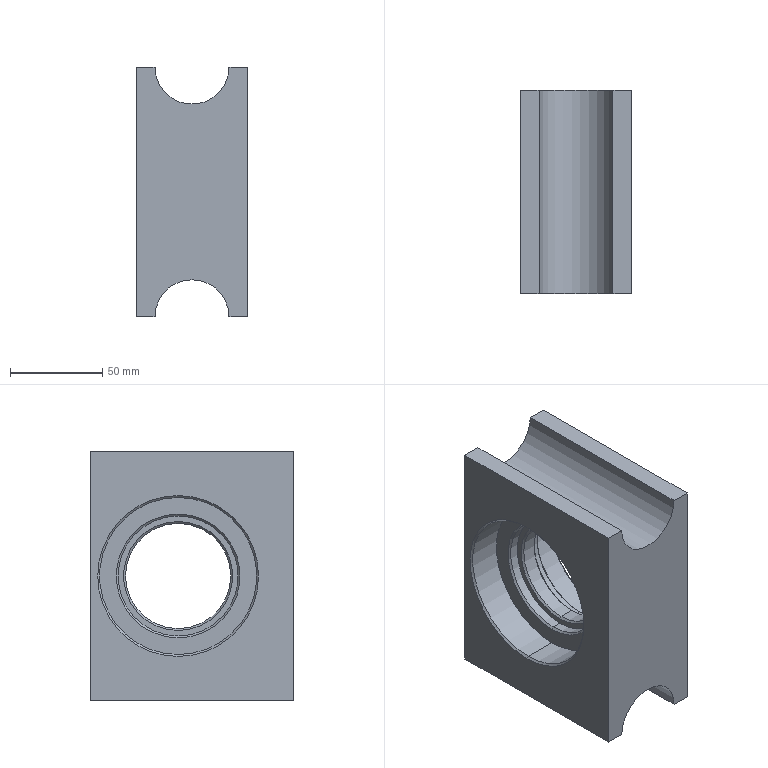Part | SolidWorks | features BaseBody 1 | 1 solid | 37 faces | box 60 x 110 x 135 mm | volume 471145 mm3 | cylinder 13 | cone 12 | plane 12 | commonest cylinder face diameters 65 x4 85 x4 40 x3 57 x2
STEP:
#1=CARTESIAN_POINT('',(0.,-55.,-47.5));
#2=VERTEX_POINT('',#1);
#3=CARTESIAN_POINT('',(20.,-55.,-67.5));
#4=VERTEX_POINT('',#3);
#5=CARTESIAN_POINT('',(0.,-55.,-67.5));
#6=DIRECTION('',(0.,1.,0.));
#7=DIRECTION('',(0.,0.,1.));
#8=AXIS2_PLACEMENT_3D('',#5,#6,#7);
#9=CIRCLE('',#8,20.);
#10=EDGE_CURVE('',#2,#4,#9,.T.);
#11=ORIENTED_EDGE('',*,*,#10,.F.);
#12=CARTESIAN_POINT('',(0.,55.,-47.5));
#13=VERTEX_POINT('',#12);
#14=CARTESIAN_POINT('',(0.,-55.,-47.5));
#15=DIRECTION('',(0.,1.,0.));
#16=VECTOR('',#15,1000.);
#17=LINE('',#14,#16);
#18=EDGE_CURVE('',#2,#13,#17,.T.);
#19=ORIENTED_EDGE('',*,*,#18,.T.);
#20=CARTESIAN_POINT('',(20.,55.,-67.5));
#21=VERTEX_POINT('',#20);
#22=CARTESIAN_POINT('',(0.,55.,-67.5));
#23=DIRECTION('',(0.,1.,0.));
#24=DIRECTION('',(0.,0.,1.));
#25=AXIS2_PLACEMENT_3D('',#22,#23,#24);
#26=CIRCLE('',#25,20.);
#27=EDGE_CURVE('',#13,#21,#26,.T.);
#28=ORIENTED_EDGE('',*,*,#27,.T.);
#29=CARTESIAN_POINT('',(20.,-55.,-67.5));
#30=DIRECTION('',(0.,1.,0.));
#31=VECTOR('',#30,1000.);
#32=LINE('',#29,#31);
#33=EDGE_CURVE('',#4,#21,#32,.T.);
#34=ORIENTED_EDGE('',*,*,#33,.F.);
#35=EDGE_LOOP('',(#11,#19,#28,#34));
#36=FACE_OUTER_BOUND('',#35,.T.);
#37=CARTESIAN_POINT('',(0.,-55.,-67.5));
#38=DIRECTION('',(0.,1.,0.));
#39=DIRECTION('',(0.,0.,1.));
#40=AXIS2_PLACEMENT_3D('',#37,#38,#39);
#41=CYLINDRICAL_SURFACE('',#40,20.);
#42=ADVANCED_FACE('',(#36),#41,.F.);
#43=CARTESIAN_POINT('',(29.,7.5,42.5));
#44=VERTEX_POINT('',#43);
#45=CARTESIAN_POINT('',(29.,7.5,-42.5));
#46=VERTEX_POINT('',#45);
#47=CARTESIAN_POINT('',(29.,7.5,0.));
#48=DIRECTION('',(1.,0.,0.));
#49=DIRECTION('',(0.,0.,-1.));
#50=AXIS2_PLACEMENT_3D('',#47,#48,#49);
#51=CIRCLE('',#50,42.5);
#52=EDGE_CURVE('',#44,#46,#51,.T.);
#53=ORIENTED_EDGE('',*,*,#52,.F.);
#54=CARTESIAN_POINT('',(30.,7.5,43.5));
#55=VERTEX_POINT('',#54);
#56=CARTESIAN_POINT('',(29.,7.5,42.5));
#57=DIRECTION('',(0.7071,0.,0.7071));
#58=VECTOR('',#57,1000.);
#59=LINE('',#56,#58);
#60=EDGE_CURVE('',#44,#55,#59,.T.);
#61=ORIENTED_EDGE('',*,*,#60,.T.);
#62=CARTESIAN_POINT('',(30.,7.5,-43.5));
#63=VERTEX_POINT('',#62);
#64=CARTESIAN_POINT('',(30.,7.5,0.));
#65=DIRECTION('',(-1.,0.,0.));
#66=DIRECTION('',(0.,0.,-1.));
#67=AXIS2_PLACEMENT_3D('',#64,#65,#66);
#68=CIRCLE('',#67,43.5);
#69=EDGE_CURVE('',#63,#55,#68,.T.);
#70=ORIENTED_EDGE('',*,*,#69,.F.);
#71=CARTESIAN_POINT('',(29.,7.5,-42.5));
#72=DIRECTION('',(0.7071,0.,-0.7071));
#73=VECTOR('',#72,1000.);
#74=LINE('',#71,#73);
#75=EDGE_CURVE('',#46,#63,#74,.T.);
#76=ORIENTED_EDGE('',*,*,#75,.F.);
#77=EDGE_LOOP('',(#53,#61,#70,#76));
#78=FACE_OUTER_BOUND('',#77,.T.);
#79=CARTESIAN_POINT('',(29.,7.5,0.));
#80=DIRECTION('',(1.,0.,0.));
#81=DIRECTION('',(0.,0.,-1.));
#82=AXIS2_PLACEMENT_3D('',#79,#80,#81);
#83=CONICAL_SURFACE('',#82,42.5,0.7854);
#84=ADVANCED_FACE('',(#78),#83,.F.);
#85=CARTESIAN_POINT('',(10.,7.5,32.5));
#86=VERTEX_POINT('',#85);
#87=CARTESIAN_POINT('',(10.,7.5,-32.5));
#88=VERTEX_POINT('',#87);
#89=CARTESIAN_POINT('',(10.,7.5,0.));
#90=DIRECTION('',(1.,0.,0.));
#91=DIRECTION('',(0.,0.,-1.));
#92=AXIS2_PLACEMENT_3D('',#89,#90,#91);
#93=CIRCLE('',#92,32.5);
#94=EDGE_CURVE('',#86,#88,#93,.T.);
#95=ORIENTED_EDGE('',*,*,#94,.F.);
#96=CARTESIAN_POINT('',(11.,7.5,33.5));
#97=VERTEX_POINT('',#96);
#98=CARTESIAN_POINT('',(10.,7.5,32.5));
#99=DIRECTION('',(0.7071,0.,0.7071));
#100=VECTOR('',#99,1000.);
#101=LINE('',#98,#100);
#102=EDGE_CURVE('',#86,#97,#101,.T.);
#103=ORIENTED_EDGE('',*,*,#102,.T.);
#104=CARTESIAN_POINT('',(11.,7.5,-33.5));
#105=VERTEX_POINT('',#104);
#106=CARTESIAN_POINT('',(11.,7.5,0.));
#107=DIRECTION('',(-1.,0.,0.));
#108=DIRECTION('',(0.,0.,-1.));
#109=AXIS2_PLACEMENT_3D('',#106,#107,#108);
#110=CIRCLE('',#109,33.5);
#111=EDGE_CURVE('',#105,#97,#110,.T.);
#112=ORIENTED_EDGE('',*,*,#111,.F.);
#113=CARTESIAN_POINT('',(10.,7.5,-32.5));
#114=DIRECTION('',(0.7071,0.,-0.7071));
#115=VECTOR('',#114,1000.);
#116=LINE('',#113,#115);
#117=EDGE_CURVE('',#88,#105,#116,.T.);
#118=ORIENTED_EDGE('',*,*,#117,.F.);
#119=EDGE_LOOP('',(#95,#103,#112,#118));
#120=FACE_OUTER_BOUND('',#119,.T.);
#121=CARTESIAN_POINT('',(10.,7.5,0.));
#122=DIRECTION('',(1.,0.,0.));
#123=DIRECTION('',(0.,0.,-1.));
#124=AXIS2_PLACEMENT_3D('',#121,#122,#123);
#125=CONICAL_SURFACE('',#124,32.5,0.7854);
#126=ADVANCED_FACE('',(#120),#125,.F.);
#127=CARTESIAN_POINT('',(4.,7.5,28.5));
#128=VERTEX_POINT('',#127);
#129=CARTESIAN_POINT('',(4.,7.5,-28.5));
#130=VERTEX_POINT('',#129);
#131=CARTESIAN_POINT('',(4.,7.5,0.));
#132=DIRECTION('',(1.,0.,0.));
#133=DIRECTION('',(0.,0.,-1.));
#134=AXIS2_PLACEMENT_3D('',#131,#132,#133);
#135=CIRCLE('',#134,28.5);
#136=EDGE_CURVE('',#128,#130,#135,.T.);
#137=ORIENTED_EDGE('',*,*,#136,.F.);
#138=CARTESIAN_POINT('',(5.,7.5,29.5));
#139=VERTEX_POINT('',#138);
#140=CARTESIAN_POINT('',(4.,7.5,28.5));
#141=DIRECTION('',(0.7071,0.,0.7071));
#142=VECTOR('',#141,1000.);
#143=LINE('',#140,#142);
#144=EDGE_CURVE('',#128,#139,#143,.T.);
#145=ORIENTED_EDGE('',*,*,#144,.T.);
#146=CARTESIAN_POINT('',(5.,7.5,-29.5));
#147=VERTEX_POINT('',#146);
#148=CARTESIAN_POINT('',(5.,7.5,0.));
#149=DIRECTION('',(-1.,0.,0.));
#150=DIRECTION('',(0.,0.,-1.));
#151=AXIS2_PLACEMENT_3D('',#148,#149,#150);
#152=CIRCLE('',#151,29.5);
#153=EDGE_CURVE('',#147,#139,#152,.T.);
#154=ORIENTED_EDGE('',*,*,#153,.F.);
#155=CARTESIAN_POINT('',(4.,7.5,-28.5));
#156=DIRECTION('',(0.7071,0.,-0.7071));
#157=VECTOR('',#156,1000.);
#158=LINE('',#155,#157);
#159=EDGE_CURVE('',#130,#147,#158,.T.);
#160=ORIENTED_EDGE('',*,*,#159,.F.);
#161=EDGE_LOOP('',(#137,#145,#154,#160));
#162=FACE_OUTER_BOUND('',#161,.T.);
#163=CARTESIAN_POINT('',(4.,7.5,0.));
#164=DIRECTION('',(1.,0.,0.));
#165=DIRECTION('',(0.,0.,-1.));
#166=AXIS2_PLACEMENT_3D('',#163,#164,#165);
#167=CONICAL_SURFACE('',#166,28.5,0.7854);
#168=ADVANCED_FACE('',(#162),#167,.F.);
#169=CARTESIAN_POINT('',(-4.,7.5,-28.5));
#170=VERTEX_POINT('',#169);
#171=CARTESIAN_POINT('',(-4.,7.5,28.5));
#172=VERTEX_POINT('',#171);
#173=CARTESIAN_POINT('',(-4.,7.5,0.));
#174=DIRECTION('',(-1.,0.,0.));
#175=DIRECTION('',(0.,0.,1.));
#176=AXIS2_PLACEMENT_3D('',#173,#174,#175);
#177=CIRCLE('',#176,28.5);
#178=EDGE_CURVE('',#170,#172,#177,.T.);
#179=ORIENTED_EDGE('',*,*,#178,.F.);
#180=CARTESIAN_POINT('',(-5.,7.5,-29.5));
#181=VERTEX_POINT('',#180);
#182=CARTESIAN_POINT('',(-4.,7.5,-28.5));
#183=DIRECTION('',(-0.7071,0.,-0.7071));
#184=VECTOR('',#183,1000.);
#185=LINE('',#182,#184);
#186=EDGE_CURVE('',#170,#181,#185,.T.);
#187=ORIENTED_EDGE('',*,*,#186,.T.);
#188=CARTESIAN_POINT('',(-5.,7.5,29.5));
#189=VERTEX_POINT('',#188);
#190=CARTESIAN_POINT('',(-5.,7.5,0.));
#191=DIRECTION('',(1.,0.,0.));
#192=DIRECTION('',(0.,0.,1.));
#193=AXIS2_PLACEMENT_3D('',#190,#191,#192);
#194=CIRCLE('',#193,29.5);
#195=EDGE_CURVE('',#189,#181,#194,.T.);
#196=ORIENTED_EDGE('',*,*,#195,.F.);
#197=CARTESIAN_POINT('',(-4.,7.5,28.5));
#198=DIRECTION('',(-0.7071,0.,0.7071));
#199=VECTOR('',#198,1000.);
#200=LINE('',#197,#199);
#201=EDGE_CURVE('',#172,#189,#200,.T.);
#202=ORIENTED_EDGE('',*,*,#201,.F.);
#203=EDGE_LOOP('',(#179,#187,#196,#202));
#204=FACE_OUTER_BOUND('',#203,.T.);
#205=CARTESIAN_POINT('',(-4.,7.5,0.));
#206=DIRECTION('',(-1.,0.,0.));
#207=DIRECTION('',(0.,0.,1.));
#208=AXIS2_PLACEMENT_3D('',#205,#206,#207);
#209=CONICAL_SURFACE('',#208,28.5,0.7854);
#210=ADVANCED_FACE('',(#204),#209,.F.);
#211=CARTESIAN_POINT('',(-10.,7.5,-32.5));
#212=VERTEX_POINT('',#211);
#213=CARTESIAN_POINT('',(-10.,7.5,32.5));
#214=VERTEX_POINT('',#213);
#215=CARTESIAN_POINT('',(-10.,7.5,0.));
#216=DIRECTION('',(-1.,0.,0.));
#217=DIRECTION('',(0.,0.,1.));
#218=AXIS2_PLACEMENT_3D('',#215,#216,#217);
#219=CIRCLE('',#218,32.5);
#220=EDGE_CURVE('',#212,#214,#219,.T.);
#221=ORIENTED_EDGE('',*,*,#220,.F.);
#222=CARTESIAN_POINT('',(-11.,7.5,-33.5));
#223=VERTEX_POINT('',#222);
#224=CARTESIAN_POINT('',(-11.,7.5,-33.5));
#225=DIRECTION('',(-0.7071,0.,-0.7071));
#226=VECTOR('',#225,1000.);
#227=LINE('',#224,#226);
#228=EDGE_CURVE('',#212,#223,#227,.T.);
#229=ORIENTED_EDGE('',*,*,#228,.T.);
#230=CARTESIAN_POINT('',(-11.,7.5,33.5));
#231=VERTEX_POINT('',#230);
#232=CARTESIAN_POINT('',(-11.,7.5,0.));
#233=DIRECTION('',(1.,0.,0.));
#234=DIRECTION('',(0.,0.,1.));
#235=AXIS2_PLACEMENT_3D('',#232,#233,#234);
#236=CIRCLE('',#235,33.5);
#237=EDGE_CURVE('',#231,#223,#236,.T.);
#238=ORIENTED_EDGE('',*,*,#237,.F.);
#239=CARTESIAN_POINT('',(-11.,7.5,33.5));
#240=DIRECTION('',(-0.7071,0.,0.7071));
#241=VECTOR('',#240,1000.);
#242=LINE('',#239,#241);
#243=EDGE_CURVE('',#214,#231,#242,.T.);
#244=ORIENTED_EDGE('',*,*,#243,.F.);
#245=EDGE_LOOP('',(#221,#229,#238,#244));
#246=FACE_OUTER_BOUND('',#245,.T.);
#247=CARTESIAN_POINT('',(-11.,7.5,0.));
#248=DIRECTION('',(-1.,0.,0.));
#249=DIRECTION('',(0.,0.,1.));
#250=AXIS2_PLACEMENT_3D('',#247,#248,#249);
#251=CONICAL_SURFACE('',#250,33.5,0.7854);
#252=ADVANCED_FACE('',(#246),#251,.F.);
#253=CARTESIAN_POINT('',(-29.,7.5,-42.5));
#254=VERTEX_POINT('',#253);
#255=CARTESIAN_POINT('',(-29.,7.5,42.5));
#256=VERTEX_POINT('',#255);
#257=CARTESIAN_POINT('',(-29.,7.5,0.));
#258=DIRECTION('',(-1.,0.,0.));
#259=DIRECTION('',(0.,0.,-1.));
#260=AXIS2_PLACEMENT_3D('',#257,#258,#259);
#261=CIRCLE('',#260,42.5);
#262=EDGE_CURVE('',#254,#256,#261,.T.);
#263=ORIENTED_EDGE('',*,*,#262,.F.);
#264=CARTESIAN_POINT('',(-30.,7.5,-43.5));
#265=VERTEX_POINT('',#264);
#266=CARTESIAN_POINT('',(-30.,7.5,-43.5));
#267=DIRECTION('',(-0.7071,0.,-0.7071));
#268=VECTOR('',#267,1000.);
#269=LINE('',#266,#268);
#270=EDGE_CURVE('',#254,#265,#269,.T.);
#271=ORIENTED_EDGE('',*,*,#270,.T.);
#272=CARTESIAN_POINT('',(-30.,7.5,43.5));
#273=VERTEX_POINT('',#272);
#274=CARTESIAN_POINT('',(-30.,7.5,0.));
#275=DIRECTION('',(1.,0.,0.));
#276=DIRECTION('',(0.,0.,-1.));
#277=AXIS2_PLACEMENT_3D('',#274,#275,#276);
#278=CIRCLE('',#277,43.5);
#279=EDGE_CURVE('',#273,#265,#278,.T.);
#280=ORIENTED_EDGE('',*,*,#279,.F.);
#281=CARTESIAN_POINT('',(-30.,7.5,43.5));
#282=DIRECTION('',(-0.7071,0.,0.7071));
#283=VECTOR('',#282,1000.);
#284=LINE('',#281,#283);
#285=EDGE_CURVE('',#256,#273,#284,.T.);
#286=ORIENTED_EDGE('',*,*,#285,.F.);
#287=EDGE_LOOP('',(#263,#271,#280,#286));
#288=FACE_OUTER_BOUND('',#287,.T.);
#289=CARTESIAN_POINT('',(-30.,7.5,0.));
#290=DIRECTION('',(-1.,0.,0.));
#291=DIRECTION('',(0.,0.,1.));
#292=AXIS2_PLACEMENT_3D('',#289,#290,#291);
#293=CONICAL_SURFACE('',#292,43.5,0.7854);
#294=ADVANCED_FACE('',(#288),#293,.F.);
#295=CARTESIAN_POINT('',(-5.,7.5,32.5));
#296=VERTEX_POINT('',#295);
#297=CARTESIAN_POINT('',(-5.,7.5,-32.5));
#298=VERTEX_POINT('',#297);
#299=CARTESIAN_POINT('',(-5.,7.5,0.));
#300=DIRECTION('',(1.,0.,0.));
#301=DIRECTION('',(0.,0.,-1.));
#302=AXIS2_PLACEMENT_3D('',#299,#300,#301);
#303=CIRCLE('',#302,32.5);
#304=EDGE_CURVE('',#296,#298,#303,.T.);
#305=ORIENTED_EDGE('',*,*,#304,.T.);
#306=CARTESIAN_POINT('',(-5.,7.5,-32.5));
#307=DIRECTION('',(-1.,0.,0.));
#308=VECTOR('',#307,1000.);
#309=LINE('',#306,#308);
#310=EDGE_CURVE('',#298,#212,#309,.T.);
#311=ORIENTED_EDGE('',*,*,#310,.T.);
#312=ORIENTED_EDGE('',*,*,#220,.T.);
#313=CARTESIAN_POINT('',(-5.,7.5,32.5));
#314=DIRECTION('',(-1.,0.,0.));
#315=VECTOR('',#314,1000.);
#316=LINE('',#313,#315);
#317=EDGE_CURVE('',#296,#214,#316,.T.);
#318=ORIENTED_EDGE('',*,*,#317,.F.);
#319=EDGE_LOOP('',(#305,#311,#312,#318));
#320=FACE_OUTER_BOUND('',#319,.T.);
#321=CARTESIAN_POINT('',(-5.,7.5,0.));
#322=DIRECTION('',(-1.,0.,0.));
#323=DIRECTION('',(0.,0.,1.));
#324=AXIS2_PLACEMENT_3D('',#321,#322,#323);
#325=CYLINDRICAL_SURFACE('',#324,32.5);
#326=ADVANCED_FACE('',(#320),#325,.F.);
#327=CARTESIAN_POINT('',(-11.,7.5,42.5));
#328=VERTEX_POINT('',#327);
#329=CARTESIAN_POINT('',(-11.,7.5,-42.5));
#330=VERTEX_POINT('',#329);
#331=CARTESIAN_POINT('',(-11.,7.5,0.));
#332=DIRECTION('',(1.,0.,0.));
#333=DIRECTION('',(0.,0.,-1.));
#334=AXIS2_PLACEMENT_3D('',#331,#332,#333);
#335=CIRCLE('',#334,42.5);
#336=EDGE_CURVE('',#328,#330,#335,.T.);
#337=ORIENTED_EDGE('',*,*,#336,.T.);
#338=CARTESIAN_POINT('',(-11.,7.5,-42.5));
#339=DIRECTION('',(-1.,0.,0.));
#340=VECTOR('',#339,1000.);
#341=LINE('',#338,#340);
#342=EDGE_CURVE('',#330,#254,#341,.T.);
#343=ORIENTED_EDGE('',*,*,#342,.T.);
#344=ORIENTED_EDGE('',*,*,#262,.T.);
#345=CARTESIAN_POINT('',(-11.,7.5,42.5));
#346=DIRECTION('',(-1.,0.,0.));
#347=VECTOR('',#346,1000.);
#348=LINE('',#345,#347);
#349=EDGE_CURVE('',#328,#256,#348,.T.);
#350=ORIENTED_EDGE('',*,*,#349,.F.);
#351=EDGE_LOOP('',(#337,#343,#344,#350));
#352=FACE_OUTER_BOUND('',#351,.T.);
#353=CARTESIAN_POINT('',(-11.,7.5,0.));
#354=DIRECTION('',(-1.,0.,0.));
#355=DIRECTION('',(0.,0.,1.));
#356=AXIS2_PLACEMENT_3D('',#353,#354,#355);
#357=CYLINDRICAL_SURFACE('',#356,42.5);
#358=ADVANCED_FACE('',(#352),#357,.F.);
#359=CARTESIAN_POINT('',(5.,7.5,32.5));
#360=VERTEX_POINT('',#359);
#361=CARTESIAN_POINT('',(5.,7.5,-32.5));
#362=VERTEX_POINT('',#361);
#363=CARTESIAN_POINT('',(5.,7.5,0.));
#364=DIRECTION('',(1.,0.,0.));
#365=DIRECTION('',(0.,0.,-1.));
#366=AXIS2_PLACEMENT_3D('',#363,#364,#365);
#367=CIRCLE('',#366,32.5);
#368=EDGE_CURVE('',#360,#362,#367,.T.);
#369=ORIENTED_EDGE('',*,*,#368,.F.);
#370=CARTESIAN_POINT('',(5.,7.5,32.5));
#371=DIRECTION('',(1.,0.,0.));
#372=VECTOR('',#371,1000.);
#373=LINE('',#370,#372);
#374=EDGE_CURVE('',#360,#86,#373,.T.);
#375=ORIENTED_EDGE('',*,*,#374,.T.);
#376=ORIENTED_EDGE('',*,*,#94,.T.);
#377=CARTESIAN_POINT('',(5.,7.5,-32.5));
#378=DIRECTION('',(1.,0.,0.));
#379=VECTOR('',#378,1000.);
#380=LINE('',#377,#379);
#381=EDGE_CURVE('',#362,#88,#380,.T.);
#382=ORIENTED_EDGE('',*,*,#381,.F.);
#383=EDGE_LOOP('',(#369,#375,#376,#382));
#384=FACE_OUTER_BOUND('',#383,.T.);
#385=CARTESIAN_POINT('',(5.,7.5,0.));
#386=DIRECTION('',(1.,0.,0.));
#387=DIRECTION('',(0.,0.,-1.));
#388=AXIS2_PLACEMENT_3D('',#385,#386,#387);
#389=CYLINDRICAL_SURFACE('',#388,32.5);
#390=ADVANCED_FACE('',(#384),#389,.F.);
#391=CARTESIAN_POINT('',(11.,7.5,42.5));
#392=VERTEX_POINT('',#391);
#393=CARTESIAN_POINT('',(11.,7.5,-42.5));
#394=VERTEX_POINT('',#393);
#395=CARTESIAN_POINT('',(11.,7.5,0.));
#396=DIRECTION('',(1.,0.,0.));
#397=DIRECTION('',(0.,0.,-1.));
#398=AXIS2_PLACEMENT_3D('',#395,#396,#397);
#399=CIRCLE('',#398,42.5);
#400=EDGE_CURVE('',#392,#394,#399,.T.);
#401=ORIENTED_EDGE('',*,*,#400,.F.);
#402=CARTESIAN_POINT('',(11.,7.5,42.5));
#403=DIRECTION('',(1.,0.,0.));
#404=VECTOR('',#403,1000.);
#405=LINE('',#402,#404);
#406=EDGE_CURVE('',#392,#44,#405,.T.);
#407=ORIENTED_EDGE('',*,*,#406,.T.);
#408=ORIENTED_EDGE('',*,*,#52,.T.);
#409=CARTESIAN_POINT('',(11.,7.5,-42.5));
#410=DIRECTION('',(1.,0.,0.));
#411=VECTOR('',#410,1000.);
#412=LINE('',#409,#411);
#413=EDGE_CURVE('',#394,#46,#412,.T.);
#414=ORIENTED_EDGE('',*,*,#413,.F.);
#415=EDGE_LOOP('',(#401,#407,#408,#414));
#416=FACE_OUTER_BOUND('',#415,.T.);
#417=CARTESIAN_POINT('',(11.,7.5,0.));
#418=DIRECTION('',(1.,0.,0.));
#419=DIRECTION('',(0.,0.,-1.));
#420=AXIS2_PLACEMENT_3D('',#417,#418,#419);
#421=CYLINDRICAL_SURFACE('',#420,42.5);
#422=ADVANCED_FACE('',(#416),#421,.F.);
#423=ORIENTED_EDGE('',*,*,#136,.T.);
#424=CARTESIAN_POINT('',(30.,7.5,-28.5));
#425=DIRECTION('',(-1.,0.,0.));
#426=VECTOR('',#425,1000.);
#427=LINE('',#424,#426);
#428=EDGE_CURVE('',#130,#170,#427,.T.);
#429=ORIENTED_EDGE('',*,*,#428,.T.);
#430=ORIENTED_EDGE('',*,*,#178,.T.);
#431=CARTESIAN_POINT('',(30.,7.5,28.5));
#432=DIRECTION('',(-1.,0.,0.));
#433=VECTOR('',#432,1000.);
#434=LINE('',#431,#433);
#435=EDGE_CURVE('',#128,#172,#434,.T.);
#436=ORIENTED_EDGE('',*,*,#435,.F.);
#437=EDGE_LOOP('',(#423,#429,#430,#436));
#438=FACE_OUTER_BOUND('',#437,.T.);
#439=CARTESIAN_POINT('',(30.,7.5,0.));
#440=DIRECTION('',(-1.,0.,0.));
#441=DIRECTION('',(0.,0.,1.));
#442=AXIS2_PLACEMENT_3D('',#439,#440,#441);
#443=CYLINDRICAL_SURFACE('',#442,28.5);
#444=ADVANCED_FACE('',(#438),#443,.F.);
#445=CARTESIAN_POINT('',(30.,-55.,-67.5));
#446=VERTEX_POINT('',#445);
#447=CARTESIAN_POINT('',(30.,-55.,-67.5));
#448=DIRECTION('',(-1.,0.,0.));
#449=VECTOR('',#448,1000.);
#450=LINE('',#447,#449);
#451=EDGE_CURVE('',#446,#4,#450,.T.);
#452=ORIENTED_EDGE('',*,*,#451,.T.);
#453=ORIENTED_EDGE('',*,*,#33,.T.);
#454=CARTESIAN_POINT('',(30.,55.,-67.5));
#455=VERTEX_POINT('',#454);
#456=CARTESIAN_POINT('',(30.,55.,-67.5));
#457=DIRECTION('',(-1.,0.,0.));
#458=VECTOR('',#457,1000.);
#459=LINE('',#456,#458);
#460=EDGE_CURVE('',#455,#21,#459,.T.);
#461=ORIENTED_EDGE('',*,*,#460,.F.);
#462=CARTESIAN_POINT('',(30.,55.,-67.5));
#463=DIRECTION('',(0.,1.,0.));
#464=VECTOR('',#463,1000.);
#465=LINE('',#462,#464);
#466=EDGE_CURVE('',#446,#455,#465,.T.);
#467=ORIENTED_EDGE('',*,*,#466,.F.);
#468=EDGE_LOOP('',(#452,#453,#461,#467));
#469=FACE_OUTER_BOUND('',#468,.T.);
#470=CARTESIAN_POINT('',(30.,55.,-67.5));
#471=DIRECTION('',(0.,0.,1.));
#472=DIRECTION('',(0.,-1.,0.));
#473=AXIS2_PLACEMENT_3D('',#470,#471,#472);
#474=PLANE('',#473);
#475=ADVANCED_FACE('',(#469),#474,.F.);
#476=CARTESIAN_POINT('',(-20.,-55.,67.5));
#477=VERTEX_POINT('',#476);
#478=CARTESIAN_POINT('',(-30.,-55.,67.5));
#479=VERTEX_POINT('',#478);
#480=CARTESIAN_POINT('',(30.,-55.,67.5));
#481=DIRECTION('',(-1.,0.,0.));
#482=VECTOR('',#481,1000.);
#483=LINE('',#480,#482);
#484=EDGE_CURVE('',#477,#479,#483,.T.);
#485=ORIENTED_EDGE('',*,*,#484,.F.);
#486=CARTESIAN_POINT('',(-20.,55.,67.5));
#487=VERTEX_POINT('',#486);
#488=CARTESIAN_POINT('',(-20.,-55.,67.5));
#489=DIRECTION('',(0.,1.,0.));
#490=VECTOR('',#489,1000.);
#491=LINE('',#488,#490);
#492=EDGE_CURVE('',#477,#487,#491,.T.);
#493=ORIENTED_EDGE('',*,*,#492,.T.);
#494=CARTESIAN_POINT('',(-30.,55.,67.5));
#495=VERTEX_POINT('',#494);
#496=CARTESIAN_POINT('',(30.,55.,67.5));
#497=DIRECTION('',(-1.,0.,0.));
#498=VECTOR('',#497,1000.);
#499=LINE('',#496,#498);
#500=EDGE_CURVE('',#487,#495,#499,.T.);
#501=ORIENTED_EDGE('',*,*,#500,.T.);
#502=CARTESIAN_POINT('',(-30.,55.,67.5));
#503=DIRECTION('',(0.,-1.,0.));
#504=VECTOR('',#503,1000.);
#505=LINE('',#502,#504);
#506=EDGE_CURVE('',#495,#479,#505,.T.);
#507=ORIENTED_EDGE('',*,*,#506,.T.);
#508=EDGE_LOOP('',(#485,#493,#501,#507));
#509=FACE_OUTER_BOUND('',#508,.T.);
#510=CARTESIAN_POINT('',(30.,55.,67.5));
#511=DIRECTION('',(0.,0.,-1.));
#512=DIRECTION('',(0.,1.,0.));
#513=AXIS2_PLACEMENT_3D('',#510,#511,#512);
#514=PLANE('',#513);
#515=ADVANCED_FACE('',(#509),#514,.F.);
#516=ORIENTED_EDGE('',*,*,#428,.F.);
#517=CARTESIAN_POINT('',(4.,7.5,0.));
#518=DIRECTION('',(1.,0.,0.));
#519=DIRECTION('',(0.,0.,-1.));
#520=AXIS2_PLACEMENT_3D('',#517,#518,#519);
#521=CIRCLE('',#520,28.5);
#522=EDGE_CURVE('',#130,#128,#521,.T.);
#523=ORIENTED_EDGE('',*,*,#522,.T.);
#524=ORIENTED_EDGE('',*,*,#435,.T.);
#525=CARTESIAN_POINT('',(-4.,7.5,0.));
#526=DIRECTION('',(-1.,0.,0.));
#527=DIRECTION('',(0.,0.,1.));
#528=AXIS2_PLACEMENT_3D('',#525,#526,#527);
#529=CIRCLE('',#528,28.5);
#530=EDGE_CURVE('',#172,#170,#529,.T.);
#531=ORIENTED_EDGE('',*,*,#530,.T.);
#532=EDGE_LOOP('',(#516,#523,#524,#531));
#533=FACE_OUTER_BOUND('',#532,.T.);
#534=CARTESIAN_POINT('',(30.,7.5,0.));
#535=DIRECTION('',(-1.,0.,0.));
#536=DIRECTION('',(0.,0.,1.));
#537=AXIS2_PLACEMENT_3D('',#534,#535,#536);
#538=CYLINDRICAL_SURFACE('',#537,28.5);
#539=ADVANCED_FACE('',(#533),#538,.F.);
#540=ORIENTED_EDGE('',*,*,#69,.T.);
#541=CARTESIAN_POINT('',(30.,7.5,0.));
#542=DIRECTION('',(-1.,0.,0.));
#543=DIRECTION('',(0.,0.,-1.));
#544=AXIS2_PLACEMENT_3D('',#541,#542,#543);
#545=CIRCLE('',#544,43.5);
#546=EDGE_CURVE('',#55,#63,#545,.T.);
#547=ORIENTED_EDGE('',*,*,#546,.T.);
#548=EDGE_LOOP('',(#540,#547));
#549=FACE_BOUND('',#548,.T.);
#550=ORIENTED_EDGE('',*,*,#466,.T.);
#551=CARTESIAN_POINT('',(30.,55.,67.5));
#552=VERTEX_POINT('',#551);
#553=CARTESIAN_POINT('',(30.,55.,67.5));
#554=DIRECTION('',(0.,0.,1.));
#555=VECTOR('',#554,1000.);
#556=LINE('',#553,#555);
#557=EDGE_CURVE('',#455,#552,#556,.T.);
#558=ORIENTED_EDGE('',*,*,#557,.T.);
#559=CARTESIAN_POINT('',(30.,-55.,67.5));
#560=VERTEX_POINT('',#559);
#561=CARTESIAN_POINT('',(30.,55.,67.5));
#562=DIRECTION('',(0.,-1.,0.));
#563=VECTOR('',#562,1000.);
#564=LINE('',#561,#563);
#565=EDGE_CURVE('',#552,#560,#564,.T.);
#566=ORIENTED_EDGE('',*,*,#565,.T.);
#567=CARTESIAN_POINT('',(30.,-55.,67.5));
#568=DIRECTION('',(0.,0.,-1.));
#569=VECTOR('',#568,1000.);
#570=LINE('',#567,#569);
#571=EDGE_CURVE('',#560,#446,#570,.T.);
#572=ORIENTED_EDGE('',*,*,#571,.T.);
#573=EDGE_LOOP('',(#550,#558,#566,#572));
#574=FACE_OUTER_BOUND('',#573,.T.);
#575=CARTESIAN_POINT('',(30.,0.,0.));
#576=DIRECTION('',(1.,0.,0.));
#577=DIRECTION('',(0.,0.,-1.));
#578=AXIS2_PLACEMENT_3D('',#575,#576,#577);
#579=PLANE('',#578);
#580=ADVANCED_FACE('',(#549,#574),#579,.T.);
#581=ORIENTED_EDGE('',*,*,#279,.T.);
#582=CARTESIAN_POINT('',(-30.,7.5,0.));
#583=DIRECTION('',(1.,0.,0.));
#584=DIRECTION('',(0.,0.,-1.));
#585=AXIS2_PLACEMENT_3D('',#582,#583,#584);
#586=CIRCLE('',#585,43.5);
#587=EDGE_CURVE('',#265,#273,#586,.T.);
#588=ORIENTED_EDGE('',*,*,#587,.T.);
#589=EDGE_LOOP('',(#581,#588));
#590=FACE_BOUND('',#589,.T.);
#591=CARTESIAN_POINT('',(-30.,-55.,-67.5));
#592=VERTEX_POINT('',#591);
#593=CARTESIAN_POINT('',(-30.,55.,-67.5));
#594=VERTEX_POINT('',#593);
#595=CARTESIAN_POINT('',(-30.,55.,-67.5));
#596=DIRECTION('',(0.,1.,0.));
#597=VECTOR('',#596,1000.);
#598=LINE('',#595,#597);
#599=EDGE_CURVE('',#592,#594,#598,.T.);
#600=ORIENTED_EDGE('',*,*,#599,.F.);
#601=CARTESIAN_POINT('',(-30.,-55.,67.5));
#602=DIRECTION('',(0.,0.,-1.));
#603=VECTOR('',#602,1000.);
#604=LINE('',#601,#603);
#605=EDGE_CURVE('',#479,#592,#604,.T.);
#606=ORIENTED_EDGE('',*,*,#605,.F.);
#607=ORIENTED_EDGE('',*,*,#506,.F.);
#608=CARTESIAN_POINT('',(-30.,55.,67.5));
#609=DIRECTION('',(0.,0.,1.));
#610=VECTOR('',#609,1000.);
#611=LINE('',#608,#610);
#612=EDGE_CURVE('',#594,#495,#611,.T.);
#613=ORIENTED_EDGE('',*,*,#612,.F.);
#614=EDGE_LOOP('',(#600,#606,#607,#613));
#615=FACE_OUTER_BOUND('',#614,.T.);
#616=CARTESIAN_POINT('',(-30.,0.,0.));
#617=DIRECTION('',(1.,0.,0.));
#618=DIRECTION('',(0.,0.,-1.));
#619=AXIS2_PLACEMENT_3D('',#616,#617,#618);
#620=PLANE('',#619);
#621=ADVANCED_FACE('',(#590,#615),#620,.F.);
#622=CARTESIAN_POINT('',(-20.,55.,-67.5));
#623=VERTEX_POINT('',#622);
#624=CARTESIAN_POINT('',(30.,55.,-67.5));
#625=DIRECTION('',(-1.,0.,0.));
#626=VECTOR('',#625,1000.);
#627=LINE('',#624,#626);
#628=EDGE_CURVE('',#623,#594,#627,.T.);
#629=ORIENTED_EDGE('',*,*,#628,.F.);
#630=CARTESIAN_POINT('',(-20.,-55.,-67.5));
#631=VERTEX_POINT('',#630);
#632=CARTESIAN_POINT('',(-20.,-55.,-67.5));
#633=DIRECTION('',(0.,-1.,0.));
#634=VECTOR('',#633,1000.);
#635=LINE('',#632,#634);
#636=EDGE_CURVE('',#623,#631,#635,.T.);
#637=ORIENTED_EDGE('',*,*,#636,.T.);
#638=CARTESIAN_POINT('',(30.,-55.,-67.5));
#639=DIRECTION('',(-1.,0.,0.));
#640=VECTOR('',#639,1000.);
#641=LINE('',#638,#640);
#642=EDGE_CURVE('',#631,#592,#641,.T.);
#643=ORIENTED_EDGE('',*,*,#642,.T.);
#644=ORIENTED_EDGE('',*,*,#599,.T.);
#645=EDGE_LOOP('',(#629,#637,#643,#644));
#646=FACE_OUTER_BOUND('',#645,.T.);
#647=CARTESIAN_POINT('',(30.,55.,-67.5));
#648=DIRECTION('',(0.,0.,1.));
#649=DIRECTION('',(0.,-1.,0.));
#650=AXIS2_PLACEMENT_3D('',#647,#648,#649);
#651=PLANE('',#650);
#652=ADVANCED_FACE('',(#646),#651,.F.);
#653=ORIENTED_EDGE('',*,*,#460,.T.);
#654=ORIENTED_EDGE('',*,*,#27,.F.);
#655=CARTESIAN_POINT('',(0.,55.,-67.5));
#656=DIRECTION('',(0.,1.,0.));
#657=DIRECTION('',(0.,0.,1.));
#658=AXIS2_PLACEMENT_3D('',#655,#656,#657);
#659=CIRCLE('',#658,20.);
#660=EDGE_CURVE('',#623,#13,#659,.T.);
#661=ORIENTED_EDGE('',*,*,#660,.F.);
#662=ORIENTED_EDGE('',*,*,#628,.T.);
#663=ORIENTED_EDGE('',*,*,#612,.T.);
#664=ORIENTED_EDGE('',*,*,#500,.F.);
#665=CARTESIAN_POINT('',(20.,55.,67.5));
#666=VERTEX_POINT('',#665);
#667=CARTESIAN_POINT('',(0.,55.,67.5));
#668=DIRECTION('',(0.,1.,0.));
#669=DIRECTION('',(0.,0.,1.));
#670=AXIS2_PLACEMENT_3D('',#667,#668,#669);
#671=CIRCLE('',#670,20.);
#672=EDGE_CURVE('',#666,#487,#671,.T.);
#673=ORIENTED_EDGE('',*,*,#672,.F.);
#674=CARTESIAN_POINT('',(30.,55.,67.5));
#675=DIRECTION('',(-1.,0.,0.));
#676=VECTOR('',#675,1000.);
#677=LINE('',#674,#676);
#678=EDGE_CURVE('',#552,#666,#677,.T.);
#679=ORIENTED_EDGE('',*,*,#678,.F.);
#680=ORIENTED_EDGE('',*,*,#557,.F.);
#681=EDGE_LOOP('',(#653,#654,#661,#662,#663,#664,#673,#679,#680));
#682=FACE_OUTER_BOUND('',#681,.T.);
#683=CARTESIAN_POINT('',(30.,55.,67.5));
#684=DIRECTION('',(0.,-1.,0.));
#685=DIRECTION('',(0.,0.,-1.));
#686=AXIS2_PLACEMENT_3D('',#683,#684,#685);
#687=PLANE('',#686);
#688=ADVANCED_FACE('',(#682),#687,.F.);
#689=ORIENTED_EDGE('',*,*,#678,.T.);
#690=CARTESIAN_POINT('',(20.,-55.,67.5));
#691=VERTEX_POINT('',#690);
#692=CARTESIAN_POINT('',(20.,-55.,67.5));
#693=DIRECTION('',(0.,-1.,0.));
#694=VECTOR('',#693,1000.);
#695=LINE('',#692,#694);
#696=EDGE_CURVE('',#666,#691,#695,.T.);
#697=ORIENTED_EDGE('',*,*,#696,.T.);
#698=CARTESIAN_POINT('',(30.,-55.,67.5));
#699=DIRECTION('',(-1.,0.,0.));
#700=VECTOR('',#699,1000.);
#701=LINE('',#698,#700);
#702=EDGE_CURVE('',#560,#691,#701,.T.);
#703=ORIENTED_EDGE('',*,*,#702,.F.);
#704=ORIENTED_EDGE('',*,*,#565,.F.);
#705=EDGE_LOOP('',(#689,#697,#703,#704));
#706=FACE_OUTER_BOUND('',#705,.T.);
#707=CARTESIAN_POINT('',(30.,55.,67.5));
#708=DIRECTION('',(0.,0.,-1.));
#709=DIRECTION('',(0.,1.,0.));
#710=AXIS2_PLACEMENT_3D('',#707,#708,#709);
#711=PLANE('',#710);
#712=ADVANCED_FACE('',(#706),#711,.F.);
#713=ORIENTED_EDGE('',*,*,#642,.F.);
#714=CARTESIAN_POINT('',(0.,-55.,-67.5));
#715=DIRECTION('',(0.,1.,0.));
#716=DIRECTION('',(0.,0.,1.));
#717=AXIS2_PLACEMENT_3D('',#714,#715,#716);
#718=CIRCLE('',#717,20.);
#719=EDGE_CURVE('',#631,#2,#718,.T.);
#720=ORIENTED_EDGE('',*,*,#719,.T.);
#721=ORIENTED_EDGE('',*,*,#10,.T.);
#722=ORIENTED_EDGE('',*,*,#451,.F.);
#723=ORIENTED_EDGE('',*,*,#571,.F.);
#724=ORIENTED_EDGE('',*,*,#702,.T.);
#725=CARTESIAN_POINT('',(0.,-55.,67.5));
#726=DIRECTION('',(0.,1.,0.));
#727=DIRECTION('',(0.,0.,1.));
#728=AXIS2_PLACEMENT_3D('',#725,#726,#727);
#729=CIRCLE('',#728,20.);
#730=EDGE_CURVE('',#691,#477,#729,.T.);
#731=ORIENTED_EDGE('',*,*,#730,.T.);
#732=ORIENTED_EDGE('',*,*,#484,.T.);
#733=ORIENTED_EDGE('',*,*,#605,.T.);
#734=EDGE_LOOP('',(#713,#720,#721,#722,#723,#724,#731,#732,#733));
#735=FACE_OUTER_BOUND('',#734,.T.);
#736=CARTESIAN_POINT('',(30.,-55.,67.5));
#737=DIRECTION('',(0.,1.,0.));
#738=DIRECTION('',(0.,0.,1.));
#739=AXIS2_PLACEMENT_3D('',#736,#737,#738);
#740=PLANE('',#739);
#741=ADVANCED_FACE('',(#735),#740,.F.);
#742=ORIENTED_EDGE('',*,*,#406,.F.);
#743=CARTESIAN_POINT('',(11.,7.5,0.));
#744=DIRECTION('',(1.,0.,0.));
#745=DIRECTION('',(0.,0.,-1.));
#746=AXIS2_PLACEMENT_3D('',#743,#744,#745);
#747=CIRCLE('',#746,42.5);
#748=EDGE_CURVE('',#394,#392,#747,.T.);
#749=ORIENTED_EDGE('',*,*,#748,.F.);
#750=ORIENTED_EDGE('',*,*,#413,.T.);
#751=CARTESIAN_POINT('',(29.,7.5,0.));
#752=DIRECTION('',(1.,0.,0.));
#753=DIRECTION('',(0.,0.,-1.));
#754=AXIS2_PLACEMENT_3D('',#751,#752,#753);
#755=CIRCLE('',#754,42.5);
#756=EDGE_CURVE('',#46,#44,#755,.T.);
#757=ORIENTED_EDGE('',*,*,#756,.T.);
#758=EDGE_LOOP('',(#742,#749,#750,#757));
#759=FACE_OUTER_BOUND('',#758,.T.);
#760=CARTESIAN_POINT('',(11.,7.5,0.));
#761=DIRECTION('',(1.,0.,0.));
#762=DIRECTION('',(0.,0.,-1.));
#763=AXIS2_PLACEMENT_3D('',#760,#761,#762);
#764=CYLINDRICAL_SURFACE('',#763,42.5);
#765=ADVANCED_FACE('',(#759),#764,.F.);
#766=ORIENTED_EDGE('',*,*,#111,.T.);
#767=CARTESIAN_POINT('',(11.,7.5,0.));
#768=DIRECTION('',(-1.,0.,0.));
#769=DIRECTION('',(0.,0.,-1.));
#770=AXIS2_PLACEMENT_3D('',#767,#768,#769);
#771=CIRCLE('',#770,33.5);
#772=EDGE_CURVE('',#97,#105,#771,.T.);
#773=ORIENTED_EDGE('',*,*,#772,.T.);
#774=EDGE_LOOP('',(#766,#773));
#775=FACE_BOUND('',#774,.T.);
#776=ORIENTED_EDGE('',*,*,#748,.T.);
#777=ORIENTED_EDGE('',*,*,#400,.T.);
#778=EDGE_LOOP('',(#776,#777));
#779=FACE_OUTER_BOUND('',#778,.T.);
#780=CARTESIAN_POINT('',(11.,7.5,0.));
#781=DIRECTION('',(1.,0.,0.));
#782=DIRECTION('',(0.,0.,-1.));
#783=AXIS2_PLACEMENT_3D('',#780,#781,#782);
#784=PLANE('',#783);
#785=ADVANCED_FACE('',(#775,#779),#784,.T.);
#786=ORIENTED_EDGE('',*,*,#374,.F.);
#787=CARTESIAN_POINT('',(5.,7.5,0.));
#788=DIRECTION('',(1.,0.,0.));
#789=DIRECTION('',(0.,0.,-1.));
#790=AXIS2_PLACEMENT_3D('',#787,#788,#789);
#791=CIRCLE('',#790,32.5);
#792=EDGE_CURVE('',#362,#360,#791,.T.);
#793=ORIENTED_EDGE('',*,*,#792,.F.);
#794=ORIENTED_EDGE('',*,*,#381,.T.);
#795=CARTESIAN_POINT('',(10.,7.5,0.));
#796=DIRECTION('',(1.,0.,0.));
#797=DIRECTION('',(0.,0.,-1.));
#798=AXIS2_PLACEMENT_3D('',#795,#796,#797);
#799=CIRCLE('',#798,32.5);
#800=EDGE_CURVE('',#88,#86,#799,.T.);
#801=ORIENTED_EDGE('',*,*,#800,.T.);
#802=EDGE_LOOP('',(#786,#793,#794,#801));
#803=FACE_OUTER_BOUND('',#802,.T.);
#804=CARTESIAN_POINT('',(5.,7.5,0.));
#805=DIRECTION('',(1.,0.,0.));
#806=DIRECTION('',(0.,0.,-1.));
#807=AXIS2_PLACEMENT_3D('',#804,#805,#806);
#808=CYLINDRICAL_SURFACE('',#807,32.5);
#809=ADVANCED_FACE('',(#803),#808,.F.);
#810=ORIENTED_EDGE('',*,*,#153,.T.);
#811=CARTESIAN_POINT('',(5.,7.5,0.));
#812=DIRECTION('',(-1.,0.,0.));
#813=DIRECTION('',(0.,0.,-1.));
#814=AXIS2_PLACEMENT_3D('',#811,#812,#813);
#815=CIRCLE('',#814,29.5);
#816=EDGE_CURVE('',#139,#147,#815,.T.);
#817=ORIENTED_EDGE('',*,*,#816,.T.);
#818=EDGE_LOOP('',(#810,#817));
#819=FACE_BOUND('',#818,.T.);
#820=ORIENTED_EDGE('',*,*,#792,.T.);
#821=ORIENTED_EDGE('',*,*,#368,.T.);
#822=EDGE_LOOP('',(#820,#821));
#823=FACE_OUTER_BOUND('',#822,.T.);
#824=CARTESIAN_POINT('',(5.,7.5,0.));
#825=DIRECTION('',(1.,0.,0.));
#826=DIRECTION('',(0.,0.,-1.));
#827=AXIS2_PLACEMENT_3D('',#824,#825,#826);
#828=PLANE('',#827);
#829=ADVANCED_FACE('',(#819,#823),#828,.T.);
#830=ORIENTED_EDGE('',*,*,#342,.F.);
#831=CARTESIAN_POINT('',(-11.,7.5,0.));
#832=DIRECTION('',(1.,0.,0.));
#833=DIRECTION('',(0.,0.,-1.));
#834=AXIS2_PLACEMENT_3D('',#831,#832,#833);
#835=CIRCLE('',#834,42.5);
#836=EDGE_CURVE('',#330,#328,#835,.T.);
#837=ORIENTED_EDGE('',*,*,#836,.T.);
#838=ORIENTED_EDGE('',*,*,#349,.T.);
#839=CARTESIAN_POINT('',(-29.,7.5,0.));
#840=DIRECTION('',(-1.,0.,0.));
#841=DIRECTION('',(0.,0.,-1.));
#842=AXIS2_PLACEMENT_3D('',#839,#840,#841);
#843=CIRCLE('',#842,42.5);
#844=EDGE_CURVE('',#256,#254,#843,.T.);
#845=ORIENTED_EDGE('',*,*,#844,.T.);
#846=EDGE_LOOP('',(#830,#837,#838,#845));
#847=FACE_OUTER_BOUND('',#846,.T.);
#848=CARTESIAN_POINT('',(-11.,7.5,0.));
#849=DIRECTION('',(-1.,0.,0.));
#850=DIRECTION('',(0.,0.,1.));
#851=AXIS2_PLACEMENT_3D('',#848,#849,#850);
#852=CYLINDRICAL_SURFACE('',#851,42.5);
#853=ADVANCED_FACE('',(#847),#852,.F.);
#854=ORIENTED_EDGE('',*,*,#237,.T.);
#855=CARTESIAN_POINT('',(-11.,7.5,0.));
#856=DIRECTION('',(1.,0.,0.));
#857=DIRECTION('',(0.,0.,1.));
#858=AXIS2_PLACEMENT_3D('',#855,#856,#857);
#859=CIRCLE('',#858,33.5);
#860=EDGE_CURVE('',#223,#231,#859,.T.);
#861=ORIENTED_EDGE('',*,*,#860,.T.);
#862=EDGE_LOOP('',(#854,#861));
#863=FACE_BOUND('',#862,.T.);
#864=ORIENTED_EDGE('',*,*,#336,.F.);
#865=ORIENTED_EDGE('',*,*,#836,.F.);
#866=EDGE_LOOP('',(#864,#865));
#867=FACE_OUTER_BOUND('',#866,.T.);
#868=CARTESIAN_POINT('',(-11.,7.5,0.));
#869=DIRECTION('',(-1.,0.,0.));
#870=DIRECTION('',(0.,0.,-1.));
#871=AXIS2_PLACEMENT_3D('',#868,#869,#870);
#872=PLANE('',#871);
#873=ADVANCED_FACE('',(#863,#867),#872,.T.);
#874=ORIENTED_EDGE('',*,*,#310,.F.);
#875=CARTESIAN_POINT('',(-5.,7.5,0.));
#876=DIRECTION('',(1.,0.,0.));
#877=DIRECTION('',(0.,0.,-1.));
#878=AXIS2_PLACEMENT_3D('',#875,#876,#877);
#879=CIRCLE('',#878,32.5);
#880=EDGE_CURVE('',#298,#296,#879,.T.);
#881=ORIENTED_EDGE('',*,*,#880,.T.);
#882=ORIENTED_EDGE('',*,*,#317,.T.);
#883=CARTESIAN_POINT('',(-10.,7.5,0.));
#884=DIRECTION('',(-1.,0.,0.));
#885=DIRECTION('',(0.,0.,1.));
#886=AXIS2_PLACEMENT_3D('',#883,#884,#885);
#887=CIRCLE('',#886,32.5);
#888=EDGE_CURVE('',#214,#212,#887,.T.);
#889=ORIENTED_EDGE('',*,*,#888,.T.);
#890=EDGE_LOOP('',(#874,#881,#882,#889));
#891=FACE_OUTER_BOUND('',#890,.T.);
#892=CARTESIAN_POINT('',(-5.,7.5,0.));
#893=DIRECTION('',(-1.,0.,0.));
#894=DIRECTION('',(0.,0.,1.));
#895=AXIS2_PLACEMENT_3D('',#892,#893,#894);
#896=CYLINDRICAL_SURFACE('',#895,32.5);
#897=ADVANCED_FACE('',(#891),#896,.F.);
#898=ORIENTED_EDGE('',*,*,#195,.T.);
#899=CARTESIAN_POINT('',(-5.,7.5,0.));
#900=DIRECTION('',(1.,0.,0.));
#901=DIRECTION('',(0.,0.,1.));
#902=AXIS2_PLACEMENT_3D('',#899,#900,#901);
#903=CIRCLE('',#902,29.5);
#904=EDGE_CURVE('',#181,#189,#903,.T.);
#905=ORIENTED_EDGE('',*,*,#904,.T.);
#906=EDGE_LOOP('',(#898,#905));
#907=FACE_BOUND('',#906,.T.);
#908=ORIENTED_EDGE('',*,*,#304,.F.);
#909=ORIENTED_EDGE('',*,*,#880,.F.);
#910=EDGE_LOOP('',(#908,#909));
#911=FACE_OUTER_BOUND('',#910,.T.);
#912=CARTESIAN_POINT('',(-5.,7.5,0.));
#913=DIRECTION('',(-1.,0.,0.));
#914=DIRECTION('',(0.,0.,-1.));
#915=AXIS2_PLACEMENT_3D('',#912,#913,#914);
#916=PLANE('',#915);
#917=ADVANCED_FACE('',(#907,#911),#916,.T.);
#918=ORIENTED_EDGE('',*,*,#270,.F.);
#919=ORIENTED_EDGE('',*,*,#844,.F.);
#920=ORIENTED_EDGE('',*,*,#285,.T.);
#921=ORIENTED_EDGE('',*,*,#587,.F.);
#922=EDGE_LOOP('',(#918,#919,#920,#921));
#923=FACE_OUTER_BOUND('',#922,.T.);
#924=CARTESIAN_POINT('',(-30.,7.5,0.));
#925=DIRECTION('',(-1.,0.,0.));
#926=DIRECTION('',(0.,0.,1.));
#927=AXIS2_PLACEMENT_3D('',#924,#925,#926);
#928=CONICAL_SURFACE('',#927,43.5,0.7854);
#929=ADVANCED_FACE('',(#923),#928,.F.);
#930=ORIENTED_EDGE('',*,*,#228,.F.);
#931=ORIENTED_EDGE('',*,*,#888,.F.);
#932=ORIENTED_EDGE('',*,*,#243,.T.);
#933=ORIENTED_EDGE('',*,*,#860,.F.);
#934=EDGE_LOOP('',(#930,#931,#932,#933));
#935=FACE_OUTER_BOUND('',#934,.T.);
#936=CARTESIAN_POINT('',(-11.,7.5,0.));
#937=DIRECTION('',(-1.,0.,0.));
#938=DIRECTION('',(0.,0.,1.));
#939=AXIS2_PLACEMENT_3D('',#936,#937,#938);
#940=CONICAL_SURFACE('',#939,33.5,0.7854);
#941=ADVANCED_FACE('',(#935),#940,.F.);
#942=ORIENTED_EDGE('',*,*,#186,.F.);
#943=ORIENTED_EDGE('',*,*,#530,.F.);
#944=ORIENTED_EDGE('',*,*,#201,.T.);
#945=ORIENTED_EDGE('',*,*,#904,.F.);
#946=EDGE_LOOP('',(#942,#943,#944,#945));
#947=FACE_OUTER_BOUND('',#946,.T.);
#948=CARTESIAN_POINT('',(-4.,7.5,0.));
#949=DIRECTION('',(-1.,0.,0.));
#950=DIRECTION('',(0.,0.,1.));
#951=AXIS2_PLACEMENT_3D('',#948,#949,#950);
#952=CONICAL_SURFACE('',#951,28.5,0.7854);
#953=ADVANCED_FACE('',(#947),#952,.F.);
#954=ORIENTED_EDGE('',*,*,#144,.F.);
#955=ORIENTED_EDGE('',*,*,#522,.F.);
#956=ORIENTED_EDGE('',*,*,#159,.T.);
#957=ORIENTED_EDGE('',*,*,#816,.F.);
#958=EDGE_LOOP('',(#954,#955,#956,#957));
#959=FACE_OUTER_BOUND('',#958,.T.);
#960=CARTESIAN_POINT('',(4.,7.5,0.));
#961=DIRECTION('',(1.,0.,0.));
#962=DIRECTION('',(0.,0.,-1.));
#963=AXIS2_PLACEMENT_3D('',#960,#961,#962);
#964=CONICAL_SURFACE('',#963,28.5,0.7854);
#965=ADVANCED_FACE('',(#959),#964,.F.);
#966=ORIENTED_EDGE('',*,*,#102,.F.);
#967=ORIENTED_EDGE('',*,*,#800,.F.);
#968=ORIENTED_EDGE('',*,*,#117,.T.);
#969=ORIENTED_EDGE('',*,*,#772,.F.);
#970=EDGE_LOOP('',(#966,#967,#968,#969));
#971=FACE_OUTER_BOUND('',#970,.T.);
#972=CARTESIAN_POINT('',(10.,7.5,0.));
#973=DIRECTION('',(1.,0.,0.));
#974=DIRECTION('',(0.,0.,-1.));
#975=AXIS2_PLACEMENT_3D('',#972,#973,#974);
#976=CONICAL_SURFACE('',#975,32.5,0.7854);
#977=ADVANCED_FACE('',(#971),#976,.F.);
#978=ORIENTED_EDGE('',*,*,#60,.F.);
#979=ORIENTED_EDGE('',*,*,#756,.F.);
#980=ORIENTED_EDGE('',*,*,#75,.T.);
#981=ORIENTED_EDGE('',*,*,#546,.F.);
#982=EDGE_LOOP('',(#978,#979,#980,#981));
#983=FACE_OUTER_BOUND('',#982,.T.);
#984=CARTESIAN_POINT('',(29.,7.5,0.));
#985=DIRECTION('',(1.,0.,0.));
#986=DIRECTION('',(0.,0.,-1.));
#987=AXIS2_PLACEMENT_3D('',#984,#985,#986);
#988=CONICAL_SURFACE('',#987,42.5,0.7854);
#989=ADVANCED_FACE('',(#983),#988,.F.);
#990=ORIENTED_EDGE('',*,*,#730,.F.);
#991=ORIENTED_EDGE('',*,*,#696,.F.);
#992=ORIENTED_EDGE('',*,*,#672,.T.);
#993=ORIENTED_EDGE('',*,*,#492,.F.);
#994=EDGE_LOOP('',(#990,#991,#992,#993));
#995=FACE_OUTER_BOUND('',#994,.T.);
#996=CARTESIAN_POINT('',(0.,-55.,67.5));
#997=DIRECTION('',(0.,1.,0.));
#998=DIRECTION('',(0.,0.,1.));
#999=AXIS2_PLACEMENT_3D('',#996,#997,#998);
#1000=CYLINDRICAL_SURFACE('',#999,20.);
#1001=ADVANCED_FACE('',(#995),#1000,.F.);
#1002=ORIENTED_EDGE('',*,*,#18,.F.);
#1003=ORIENTED_EDGE('',*,*,#719,.F.);
#1004=ORIENTED_EDGE('',*,*,#636,.F.);
#1005=ORIENTED_EDGE('',*,*,#660,.T.);
#1006=EDGE_LOOP('',(#1002,#1003,#1004,#1005));
#1007=FACE_OUTER_BOUND('',#1006,.T.);
#1008=CARTESIAN_POINT('',(0.,-55.,-67.5));
#1009=DIRECTION('',(0.,1.,0.));
#1010=DIRECTION('',(0.,0.,1.));
#1011=AXIS2_PLACEMENT_3D('',#1008,#1009,#1010);
#1012=CYLINDRICAL_SURFACE('',#1011,20.);
#1013=ADVANCED_FACE('',(#1007),#1012,.F.);
#1014=CLOSED_SHELL('',(#42,#84,#126,#168,#210,#252,#294,#326,#358,#390,#422,#444,#475,#515,#539,#580,#621,#652,#688,#712,#741,#765,#785,#809,#829,#853,#873,#897,#917,#929,#941,#953,#965,#977,#989,#1001,#1013));
#1015=MANIFOLD_SOLID_BREP('',#1014);
#1016=CARTESIAN_POINT('',(0.,0.,0.));
#1017=DIRECTION('',(0.,0.,1.));
#1018=DIRECTION('',(1.,0.,0.));
#1019=AXIS2_PLACEMENT_3D('',#1016,#1017,#1018);
#1020=(LENGTH_UNIT()NAMED_UNIT(*)SI_UNIT(.MILLI.,.METRE.));
#1021=UNCERTAINTY_MEASURE_WITH_UNIT(LENGTH_MEASURE(0.00001),#1020,'','');
#1022=(NAMED_UNIT(*)PLANE_ANGLE_UNIT()SI_UNIT($,.RADIAN.));
#1023=(NAMED_UNIT(*)SI_UNIT($,.STERADIAN.)SOLID_ANGLE_UNIT());
#1024=(GEOMETRIC_REPRESENTATION_CONTEXT(3)GLOBAL_UNCERTAINTY_ASSIGNED_CONTEXT((#1021))GLOBAL_UNIT_ASSIGNED_CONTEXT((#1020,#1022,#1023))REPRESENTATION_CONTEXT('',''));
#1025=ADVANCED_BREP_SHAPE_REPRESENTATION('',(#1015,#1019),#1024);